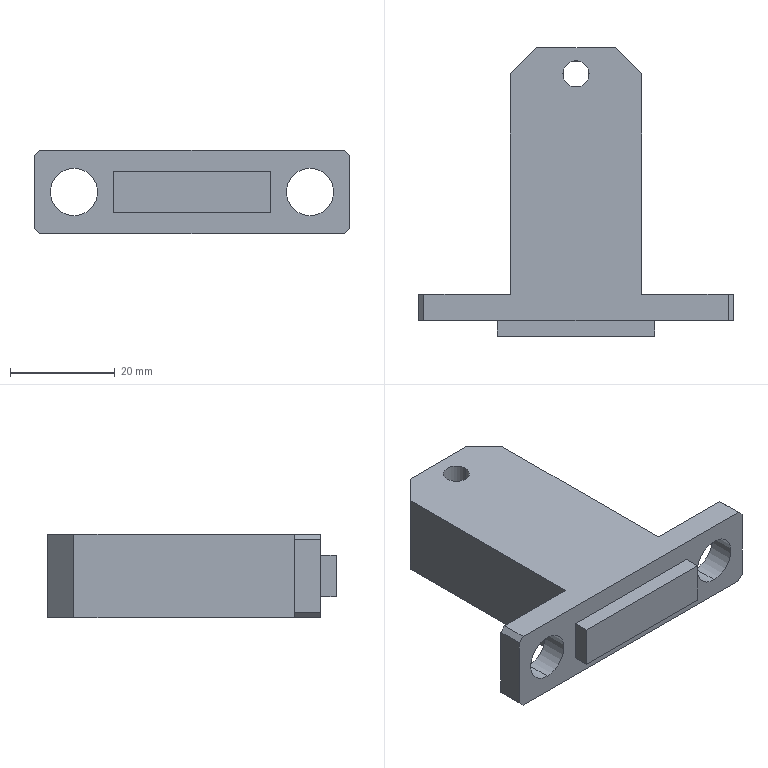Part | SolidWorks | features BaseBody 1 | 1 solid | 27 faces | box 60 x 55 x 16 mm | volume 22960 mm3 | plane 21 | cylinder 6 | commonest cylinder face diameters 9 x4 5 x2
STEP:
#1=CARTESIAN_POINT('',(-2.5,50.,-8.));
#2=VERTEX_POINT('',#1);
#3=CARTESIAN_POINT('',(2.5,50.,-8.));
#4=VERTEX_POINT('',#3);
#5=CARTESIAN_POINT('',(0.,50.,-8.));
#6=DIRECTION('',(0.,0.,1.));
#7=DIRECTION('',(1.,0.,0.));
#8=AXIS2_PLACEMENT_3D('',#5,#6,#7);
#9=CIRCLE('',#8,2.5);
#10=EDGE_CURVE('',#2,#4,#9,.T.);
#11=ORIENTED_EDGE('',*,*,#10,.F.);
#12=CARTESIAN_POINT('',(-2.5,50.,8.));
#13=VERTEX_POINT('',#12);
#14=CARTESIAN_POINT('',(-2.5,50.,8.));
#15=DIRECTION('',(0.,0.,1.));
#16=VECTOR('',#15,1000.);
#17=LINE('',#14,#16);
#18=EDGE_CURVE('',#2,#13,#17,.T.);
#19=ORIENTED_EDGE('',*,*,#18,.T.);
#20=CARTESIAN_POINT('',(2.5,50.,8.));
#21=VERTEX_POINT('',#20);
#22=CARTESIAN_POINT('',(0.,50.,8.));
#23=DIRECTION('',(0.,0.,1.));
#24=DIRECTION('',(1.,0.,0.));
#25=AXIS2_PLACEMENT_3D('',#22,#23,#24);
#26=CIRCLE('',#25,2.5);
#27=EDGE_CURVE('',#13,#21,#26,.T.);
#28=ORIENTED_EDGE('',*,*,#27,.T.);
#29=CARTESIAN_POINT('',(2.5,50.,8.));
#30=DIRECTION('',(0.,0.,1.));
#31=VECTOR('',#30,1000.);
#32=LINE('',#29,#31);
#33=EDGE_CURVE('',#4,#21,#32,.T.);
#34=ORIENTED_EDGE('',*,*,#33,.F.);
#35=EDGE_LOOP('',(#11,#19,#28,#34));
#36=FACE_OUTER_BOUND('',#35,.T.);
#37=CARTESIAN_POINT('',(0.,50.,8.));
#38=DIRECTION('',(0.,0.,1.));
#39=DIRECTION('',(1.,0.,0.));
#40=AXIS2_PLACEMENT_3D('',#37,#38,#39);
#41=CYLINDRICAL_SURFACE('',#40,2.5);
#42=ADVANCED_FACE('',(#36),#41,.F.);
#43=CARTESIAN_POINT('',(-22.5,3.,4.5));
#44=VERTEX_POINT('',#43);
#45=CARTESIAN_POINT('',(-22.5,3.,-4.5));
#46=VERTEX_POINT('',#45);
#47=CARTESIAN_POINT('',(-22.5,3.,0.));
#48=DIRECTION('',(0.,-1.,0.));
#49=DIRECTION('',(0.,0.,-1.));
#50=AXIS2_PLACEMENT_3D('',#47,#48,#49);
#51=CIRCLE('',#50,4.5);
#52=EDGE_CURVE('',#44,#46,#51,.T.);
#53=ORIENTED_EDGE('',*,*,#52,.T.);
#54=CARTESIAN_POINT('',(-22.5,8.,-4.5));
#55=VERTEX_POINT('',#54);
#56=CARTESIAN_POINT('',(-22.5,8.,-4.5));
#57=DIRECTION('',(0.,1.,0.));
#58=VECTOR('',#57,1000.);
#59=LINE('',#56,#58);
#60=EDGE_CURVE('',#46,#55,#59,.T.);
#61=ORIENTED_EDGE('',*,*,#60,.T.);
#62=CARTESIAN_POINT('',(-22.5,8.,4.5));
#63=VERTEX_POINT('',#62);
#64=CARTESIAN_POINT('',(-22.5,8.,0.));
#65=DIRECTION('',(0.,1.,0.));
#66=DIRECTION('',(0.,0.,1.));
#67=AXIS2_PLACEMENT_3D('',#64,#65,#66);
#68=CIRCLE('',#67,4.5);
#69=EDGE_CURVE('',#55,#63,#68,.T.);
#70=ORIENTED_EDGE('',*,*,#69,.T.);
#71=CARTESIAN_POINT('',(-22.5,8.,4.5));
#72=DIRECTION('',(0.,1.,0.));
#73=VECTOR('',#72,1000.);
#74=LINE('',#71,#73);
#75=EDGE_CURVE('',#44,#63,#74,.T.);
#76=ORIENTED_EDGE('',*,*,#75,.F.);
#77=EDGE_LOOP('',(#53,#61,#70,#76));
#78=FACE_OUTER_BOUND('',#77,.T.);
#79=CARTESIAN_POINT('',(-22.5,8.,0.));
#80=DIRECTION('',(0.,1.,0.));
#81=DIRECTION('',(0.,0.,1.));
#82=AXIS2_PLACEMENT_3D('',#79,#80,#81);
#83=CYLINDRICAL_SURFACE('',#82,4.5);
#84=ADVANCED_FACE('',(#78),#83,.F.);
#85=CARTESIAN_POINT('',(22.5,3.,4.5));
#86=VERTEX_POINT('',#85);
#87=CARTESIAN_POINT('',(22.5,3.,-4.5));
#88=VERTEX_POINT('',#87);
#89=CARTESIAN_POINT('',(22.5,3.,0.));
#90=DIRECTION('',(0.,-1.,0.));
#91=DIRECTION('',(0.,0.,-1.));
#92=AXIS2_PLACEMENT_3D('',#89,#90,#91);
#93=CIRCLE('',#92,4.5);
#94=EDGE_CURVE('',#86,#88,#93,.T.);
#95=ORIENTED_EDGE('',*,*,#94,.T.);
#96=CARTESIAN_POINT('',(22.5,8.,-4.5));
#97=VERTEX_POINT('',#96);
#98=CARTESIAN_POINT('',(22.5,8.,-4.5));
#99=DIRECTION('',(0.,1.,0.));
#100=VECTOR('',#99,1000.);
#101=LINE('',#98,#100);
#102=EDGE_CURVE('',#88,#97,#101,.T.);
#103=ORIENTED_EDGE('',*,*,#102,.T.);
#104=CARTESIAN_POINT('',(22.5,8.,4.5));
#105=VERTEX_POINT('',#104);
#106=CARTESIAN_POINT('',(22.5,8.,0.));
#107=DIRECTION('',(0.,1.,0.));
#108=DIRECTION('',(0.,0.,1.));
#109=AXIS2_PLACEMENT_3D('',#106,#107,#108);
#110=CIRCLE('',#109,4.5);
#111=EDGE_CURVE('',#97,#105,#110,.T.);
#112=ORIENTED_EDGE('',*,*,#111,.T.);
#113=CARTESIAN_POINT('',(22.5,8.,4.5));
#114=DIRECTION('',(0.,1.,0.));
#115=VECTOR('',#114,1000.);
#116=LINE('',#113,#115);
#117=EDGE_CURVE('',#86,#105,#116,.T.);
#118=ORIENTED_EDGE('',*,*,#117,.F.);
#119=EDGE_LOOP('',(#95,#103,#112,#118));
#120=FACE_OUTER_BOUND('',#119,.T.);
#121=CARTESIAN_POINT('',(22.5,8.,0.));
#122=DIRECTION('',(0.,1.,0.));
#123=DIRECTION('',(0.,0.,1.));
#124=AXIS2_PLACEMENT_3D('',#121,#122,#123);
#125=CYLINDRICAL_SURFACE('',#124,4.5);
#126=ADVANCED_FACE('',(#120),#125,.F.);
#127=CARTESIAN_POINT('',(29.,3.,8.));
#128=VERTEX_POINT('',#127);
#129=CARTESIAN_POINT('',(-29.,3.,8.));
#130=VERTEX_POINT('',#129);
#131=CARTESIAN_POINT('',(-30.,3.,8.));
#132=DIRECTION('',(-1.,0.,0.));
#133=VECTOR('',#132,1000.);
#134=LINE('',#131,#133);
#135=EDGE_CURVE('',#128,#130,#134,.T.);
#136=ORIENTED_EDGE('',*,*,#135,.F.);
#137=CARTESIAN_POINT('',(29.,8.,8.));
#138=VERTEX_POINT('',#137);
#139=CARTESIAN_POINT('',(29.,55.,8.));
#140=DIRECTION('',(0.,1.,0.));
#141=VECTOR('',#140,1000.);
#142=LINE('',#139,#141);
#143=EDGE_CURVE('',#128,#138,#142,.T.);
#144=ORIENTED_EDGE('',*,*,#143,.T.);
#145=CARTESIAN_POINT('',(12.5,8.,8.));
#146=VERTEX_POINT('',#145);
#147=CARTESIAN_POINT('',(30.,8.,8.));
#148=DIRECTION('',(1.,0.,0.));
#149=VECTOR('',#148,1000.);
#150=LINE('',#147,#149);
#151=EDGE_CURVE('',#146,#138,#150,.T.);
#152=ORIENTED_EDGE('',*,*,#151,.F.);
#153=CARTESIAN_POINT('',(12.5,50.,8.));
#154=VERTEX_POINT('',#153);
#155=CARTESIAN_POINT('',(12.5,55.,8.));
#156=DIRECTION('',(0.,-1.,0.));
#157=VECTOR('',#156,1000.);
#158=LINE('',#155,#157);
#159=EDGE_CURVE('',#154,#146,#158,.T.);
#160=ORIENTED_EDGE('',*,*,#159,.F.);
#161=CARTESIAN_POINT('',(7.5,55.,8.));
#162=VERTEX_POINT('',#161);
#163=CARTESIAN_POINT('',(12.5,50.,8.));
#164=DIRECTION('',(-0.7071,0.7071,0.));
#165=VECTOR('',#164,1000.);
#166=LINE('',#163,#165);
#167=EDGE_CURVE('',#154,#162,#166,.T.);
#168=ORIENTED_EDGE('',*,*,#167,.T.);
#169=CARTESIAN_POINT('',(-7.5,55.,8.));
#170=VERTEX_POINT('',#169);
#171=CARTESIAN_POINT('',(30.,55.,8.));
#172=DIRECTION('',(1.,0.,0.));
#173=VECTOR('',#172,1000.);
#174=LINE('',#171,#173);
#175=EDGE_CURVE('',#170,#162,#174,.T.);
#176=ORIENTED_EDGE('',*,*,#175,.F.);
#177=CARTESIAN_POINT('',(-12.5,50.,8.));
#178=VERTEX_POINT('',#177);
#179=CARTESIAN_POINT('',(-7.5,55.,8.));
#180=DIRECTION('',(-0.7071,-0.7071,0.));
#181=VECTOR('',#180,1000.);
#182=LINE('',#179,#181);
#183=EDGE_CURVE('',#170,#178,#182,.T.);
#184=ORIENTED_EDGE('',*,*,#183,.T.);
#185=CARTESIAN_POINT('',(-12.5,8.,8.));
#186=VERTEX_POINT('',#185);
#187=CARTESIAN_POINT('',(-12.5,55.,8.));
#188=DIRECTION('',(0.,1.,0.));
#189=VECTOR('',#188,1000.);
#190=LINE('',#187,#189);
#191=EDGE_CURVE('',#186,#178,#190,.T.);
#192=ORIENTED_EDGE('',*,*,#191,.F.);
#193=CARTESIAN_POINT('',(-29.,8.,8.));
#194=VERTEX_POINT('',#193);
#195=CARTESIAN_POINT('',(-30.,8.,8.));
#196=DIRECTION('',(1.,0.,0.));
#197=VECTOR('',#196,1000.);
#198=LINE('',#195,#197);
#199=EDGE_CURVE('',#194,#186,#198,.T.);
#200=ORIENTED_EDGE('',*,*,#199,.F.);
#201=CARTESIAN_POINT('',(-29.,55.,8.));
#202=DIRECTION('',(0.,-1.,0.));
#203=VECTOR('',#202,1000.);
#204=LINE('',#201,#203);
#205=EDGE_CURVE('',#194,#130,#204,.T.);
#206=ORIENTED_EDGE('',*,*,#205,.T.);
#207=EDGE_LOOP('',(#136,#144,#152,#160,#168,#176,#184,#192,#200,#206));
#208=FACE_OUTER_BOUND('',#207,.T.);
#209=CARTESIAN_POINT('',(0.,50.,8.));
#210=DIRECTION('',(0.,0.,1.));
#211=DIRECTION('',(1.,0.,0.));
#212=AXIS2_PLACEMENT_3D('',#209,#210,#211);
#213=CIRCLE('',#212,2.5);
#214=EDGE_CURVE('',#21,#13,#213,.T.);
#215=ORIENTED_EDGE('',*,*,#214,.F.);
#216=ORIENTED_EDGE('',*,*,#27,.F.);
#217=EDGE_LOOP('',(#215,#216));
#218=FACE_BOUND('',#217,.T.);
#219=CARTESIAN_POINT('',(30.,55.,8.));
#220=DIRECTION('',(0.,0.,-1.));
#221=DIRECTION('',(-1.,0.,0.));
#222=AXIS2_PLACEMENT_3D('',#219,#220,#221);
#223=PLANE('',#222);
#224=ADVANCED_FACE('',(#208,#218),#223,.F.);
#225=CARTESIAN_POINT('',(30.,3.,-7.));
#226=VERTEX_POINT('',#225);
#227=CARTESIAN_POINT('',(30.,3.,7.));
#228=VERTEX_POINT('',#227);
#229=CARTESIAN_POINT('',(30.,3.,8.));
#230=DIRECTION('',(0.,0.,1.));
#231=VECTOR('',#230,1000.);
#232=LINE('',#229,#231);
#233=EDGE_CURVE('',#226,#228,#232,.T.);
#234=ORIENTED_EDGE('',*,*,#233,.F.);
#235=CARTESIAN_POINT('',(30.,8.,-7.));
#236=VERTEX_POINT('',#235);
#237=CARTESIAN_POINT('',(30.,55.,-7.));
#238=DIRECTION('',(0.,1.,0.));
#239=VECTOR('',#238,1000.);
#240=LINE('',#237,#239);
#241=EDGE_CURVE('',#226,#236,#240,.T.);
#242=ORIENTED_EDGE('',*,*,#241,.T.);
#243=CARTESIAN_POINT('',(30.,8.,7.));
#244=VERTEX_POINT('',#243);
#245=CARTESIAN_POINT('',(30.,8.,-8.));
#246=DIRECTION('',(0.,0.,1.));
#247=VECTOR('',#246,1000.);
#248=LINE('',#245,#247);
#249=EDGE_CURVE('',#236,#244,#248,.T.);
#250=ORIENTED_EDGE('',*,*,#249,.T.);
#251=CARTESIAN_POINT('',(30.,55.,7.));
#252=DIRECTION('',(0.,-1.,0.));
#253=VECTOR('',#252,1000.);
#254=LINE('',#251,#253);
#255=EDGE_CURVE('',#244,#228,#254,.T.);
#256=ORIENTED_EDGE('',*,*,#255,.T.);
#257=EDGE_LOOP('',(#234,#242,#250,#256));
#258=FACE_OUTER_BOUND('',#257,.T.);
#259=CARTESIAN_POINT('',(30.,55.,-8.));
#260=DIRECTION('',(-1.,0.,0.));
#261=DIRECTION('',(0.,0.,1.));
#262=AXIS2_PLACEMENT_3D('',#259,#260,#261);
#263=PLANE('',#262);
#264=ADVANCED_FACE('',(#258),#263,.F.);
#265=ORIENTED_EDGE('',*,*,#102,.F.);
#266=CARTESIAN_POINT('',(22.5,3.,0.));
#267=DIRECTION('',(0.,-1.,0.));
#268=DIRECTION('',(0.,0.,-1.));
#269=AXIS2_PLACEMENT_3D('',#266,#267,#268);
#270=CIRCLE('',#269,4.5);
#271=EDGE_CURVE('',#88,#86,#270,.T.);
#272=ORIENTED_EDGE('',*,*,#271,.T.);
#273=ORIENTED_EDGE('',*,*,#117,.T.);
#274=CARTESIAN_POINT('',(22.5,8.,0.));
#275=DIRECTION('',(0.,1.,0.));
#276=DIRECTION('',(0.,0.,1.));
#277=AXIS2_PLACEMENT_3D('',#274,#275,#276);
#278=CIRCLE('',#277,4.5);
#279=EDGE_CURVE('',#105,#97,#278,.T.);
#280=ORIENTED_EDGE('',*,*,#279,.T.);
#281=EDGE_LOOP('',(#265,#272,#273,#280));
#282=FACE_OUTER_BOUND('',#281,.T.);
#283=CARTESIAN_POINT('',(22.5,8.,0.));
#284=DIRECTION('',(0.,1.,0.));
#285=DIRECTION('',(0.,0.,1.));
#286=AXIS2_PLACEMENT_3D('',#283,#284,#285);
#287=CYLINDRICAL_SURFACE('',#286,4.5);
#288=ADVANCED_FACE('',(#282),#287,.F.);
#289=CARTESIAN_POINT('',(-30.,3.,7.));
#290=VERTEX_POINT('',#289);
#291=CARTESIAN_POINT('',(-30.,3.,-7.));
#292=VERTEX_POINT('',#291);
#293=CARTESIAN_POINT('',(-30.,3.,-8.));
#294=DIRECTION('',(0.,0.,-1.));
#295=VECTOR('',#294,1000.);
#296=LINE('',#293,#295);
#297=EDGE_CURVE('',#290,#292,#296,.T.);
#298=ORIENTED_EDGE('',*,*,#297,.F.);
#299=CARTESIAN_POINT('',(-30.,8.,7.));
#300=VERTEX_POINT('',#299);
#301=CARTESIAN_POINT('',(-30.,55.,7.));
#302=DIRECTION('',(0.,1.,0.));
#303=VECTOR('',#302,1000.);
#304=LINE('',#301,#303);
#305=EDGE_CURVE('',#290,#300,#304,.T.);
#306=ORIENTED_EDGE('',*,*,#305,.T.);
#307=CARTESIAN_POINT('',(-30.,8.,-7.));
#308=VERTEX_POINT('',#307);
#309=CARTESIAN_POINT('',(-30.,8.,-8.));
#310=DIRECTION('',(0.,0.,1.));
#311=VECTOR('',#310,1000.);
#312=LINE('',#309,#311);
#313=EDGE_CURVE('',#308,#300,#312,.T.);
#314=ORIENTED_EDGE('',*,*,#313,.F.);
#315=CARTESIAN_POINT('',(-30.,55.,-7.));
#316=DIRECTION('',(0.,-1.,0.));
#317=VECTOR('',#316,1000.);
#318=LINE('',#315,#317);
#319=EDGE_CURVE('',#308,#292,#318,.T.);
#320=ORIENTED_EDGE('',*,*,#319,.T.);
#321=EDGE_LOOP('',(#298,#306,#314,#320));
#322=FACE_OUTER_BOUND('',#321,.T.);
#323=CARTESIAN_POINT('',(-30.,55.,-8.));
#324=DIRECTION('',(1.,0.,0.));
#325=DIRECTION('',(0.,0.,-1.));
#326=AXIS2_PLACEMENT_3D('',#323,#324,#325);
#327=PLANE('',#326);
#328=ADVANCED_FACE('',(#322),#327,.F.);
#329=ORIENTED_EDGE('',*,*,#60,.F.);
#330=CARTESIAN_POINT('',(-22.5,3.,0.));
#331=DIRECTION('',(0.,-1.,0.));
#332=DIRECTION('',(0.,0.,-1.));
#333=AXIS2_PLACEMENT_3D('',#330,#331,#332);
#334=CIRCLE('',#333,4.5);
#335=EDGE_CURVE('',#46,#44,#334,.T.);
#336=ORIENTED_EDGE('',*,*,#335,.T.);
#337=ORIENTED_EDGE('',*,*,#75,.T.);
#338=CARTESIAN_POINT('',(-22.5,8.,0.));
#339=DIRECTION('',(0.,1.,0.));
#340=DIRECTION('',(0.,0.,1.));
#341=AXIS2_PLACEMENT_3D('',#338,#339,#340);
#342=CIRCLE('',#341,4.5);
#343=EDGE_CURVE('',#63,#55,#342,.T.);
#344=ORIENTED_EDGE('',*,*,#343,.T.);
#345=EDGE_LOOP('',(#329,#336,#337,#344));
#346=FACE_OUTER_BOUND('',#345,.T.);
#347=CARTESIAN_POINT('',(-22.5,8.,0.));
#348=DIRECTION('',(0.,1.,0.));
#349=DIRECTION('',(0.,0.,1.));
#350=AXIS2_PLACEMENT_3D('',#347,#348,#349);
#351=CYLINDRICAL_SURFACE('',#350,4.5);
#352=ADVANCED_FACE('',(#346),#351,.F.);
#353=CARTESIAN_POINT('',(15.,0.,4.));
#354=VERTEX_POINT('',#353);
#355=CARTESIAN_POINT('',(15.,0.,-4.));
#356=VERTEX_POINT('',#355);
#357=CARTESIAN_POINT('',(15.,0.,8.));
#358=DIRECTION('',(0.,0.,-1.));
#359=VECTOR('',#358,1000.);
#360=LINE('',#357,#359);
#361=EDGE_CURVE('',#354,#356,#360,.T.);
#362=ORIENTED_EDGE('',*,*,#361,.F.);
#363=CARTESIAN_POINT('',(-15.,0.,4.));
#364=VERTEX_POINT('',#363);
#365=CARTESIAN_POINT('',(-30.,0.,4.));
#366=DIRECTION('',(1.,0.,0.));
#367=VECTOR('',#366,1000.);
#368=LINE('',#365,#367);
#369=EDGE_CURVE('',#364,#354,#368,.T.);
#370=ORIENTED_EDGE('',*,*,#369,.F.);
#371=CARTESIAN_POINT('',(-15.,0.,-4.));
#372=VERTEX_POINT('',#371);
#373=CARTESIAN_POINT('',(-15.,0.,8.));
#374=DIRECTION('',(0.,0.,1.));
#375=VECTOR('',#374,1000.);
#376=LINE('',#373,#375);
#377=EDGE_CURVE('',#372,#364,#376,.T.);
#378=ORIENTED_EDGE('',*,*,#377,.F.);
#379=CARTESIAN_POINT('',(-30.,0.,-4.));
#380=DIRECTION('',(-1.,0.,0.));
#381=VECTOR('',#380,1000.);
#382=LINE('',#379,#381);
#383=EDGE_CURVE('',#356,#372,#382,.T.);
#384=ORIENTED_EDGE('',*,*,#383,.F.);
#385=EDGE_LOOP('',(#362,#370,#378,#384));
#386=FACE_OUTER_BOUND('',#385,.T.);
#387=CARTESIAN_POINT('',(0.,0.,0.));
#388=DIRECTION('',(0.,-1.,0.));
#389=DIRECTION('',(0.,0.,-1.));
#390=AXIS2_PLACEMENT_3D('',#387,#388,#389);
#391=PLANE('',#390);
#392=ADVANCED_FACE('',(#386),#391,.T.);
#393=CARTESIAN_POINT('',(15.,3.,-4.));
#394=VERTEX_POINT('',#393);
#395=CARTESIAN_POINT('',(-15.,3.,-4.));
#396=VERTEX_POINT('',#395);
#397=CARTESIAN_POINT('',(-30.,3.,-4.));
#398=DIRECTION('',(-1.,0.,0.));
#399=VECTOR('',#398,1000.);
#400=LINE('',#397,#399);
#401=EDGE_CURVE('',#394,#396,#400,.T.);
#402=ORIENTED_EDGE('',*,*,#401,.F.);
#403=CARTESIAN_POINT('',(15.,3.,-4.));
#404=DIRECTION('',(0.,-1.,0.));
#405=VECTOR('',#404,1000.);
#406=LINE('',#403,#405);
#407=EDGE_CURVE('',#394,#356,#406,.T.);
#408=ORIENTED_EDGE('',*,*,#407,.T.);
#409=ORIENTED_EDGE('',*,*,#383,.T.);
#410=CARTESIAN_POINT('',(-15.,3.,-4.));
#411=DIRECTION('',(0.,1.,0.));
#412=VECTOR('',#411,1000.);
#413=LINE('',#410,#412);
#414=EDGE_CURVE('',#372,#396,#413,.T.);
#415=ORIENTED_EDGE('',*,*,#414,.T.);
#416=EDGE_LOOP('',(#402,#408,#409,#415));
#417=FACE_OUTER_BOUND('',#416,.T.);
#418=CARTESIAN_POINT('',(-30.,3.,-4.));
#419=DIRECTION('',(0.,0.,1.));
#420=DIRECTION('',(1.,0.,0.));
#421=AXIS2_PLACEMENT_3D('',#418,#419,#420);
#422=PLANE('',#421);
#423=ADVANCED_FACE('',(#417),#422,.F.);
#424=ORIENTED_EDGE('',*,*,#369,.T.);
#425=CARTESIAN_POINT('',(15.,3.,4.));
#426=VERTEX_POINT('',#425);
#427=CARTESIAN_POINT('',(15.,3.,4.));
#428=DIRECTION('',(0.,1.,0.));
#429=VECTOR('',#428,1000.);
#430=LINE('',#427,#429);
#431=EDGE_CURVE('',#354,#426,#430,.T.);
#432=ORIENTED_EDGE('',*,*,#431,.T.);
#433=CARTESIAN_POINT('',(-15.,3.,4.));
#434=VERTEX_POINT('',#433);
#435=CARTESIAN_POINT('',(-30.,3.,4.));
#436=DIRECTION('',(1.,0.,0.));
#437=VECTOR('',#436,1000.);
#438=LINE('',#435,#437);
#439=EDGE_CURVE('',#434,#426,#438,.T.);
#440=ORIENTED_EDGE('',*,*,#439,.F.);
#441=CARTESIAN_POINT('',(-15.,3.,4.));
#442=DIRECTION('',(0.,-1.,0.));
#443=VECTOR('',#442,1000.);
#444=LINE('',#441,#443);
#445=EDGE_CURVE('',#434,#364,#444,.T.);
#446=ORIENTED_EDGE('',*,*,#445,.T.);
#447=EDGE_LOOP('',(#424,#432,#440,#446));
#448=FACE_OUTER_BOUND('',#447,.T.);
#449=CARTESIAN_POINT('',(-30.,3.,4.));
#450=DIRECTION('',(0.,0.,-1.));
#451=DIRECTION('',(-1.,0.,0.));
#452=AXIS2_PLACEMENT_3D('',#449,#450,#451);
#453=PLANE('',#452);
#454=ADVANCED_FACE('',(#448),#453,.F.);
#455=CARTESIAN_POINT('',(0.,50.,-8.));
#456=DIRECTION('',(0.,0.,1.));
#457=DIRECTION('',(1.,0.,0.));
#458=AXIS2_PLACEMENT_3D('',#455,#456,#457);
#459=CIRCLE('',#458,2.5);
#460=EDGE_CURVE('',#4,#2,#459,.T.);
#461=ORIENTED_EDGE('',*,*,#460,.T.);
#462=ORIENTED_EDGE('',*,*,#10,.T.);
#463=EDGE_LOOP('',(#461,#462));
#464=FACE_BOUND('',#463,.T.);
#465=CARTESIAN_POINT('',(12.5,8.,-8.));
#466=VERTEX_POINT('',#465);
#467=CARTESIAN_POINT('',(29.,8.,-8.));
#468=VERTEX_POINT('',#467);
#469=CARTESIAN_POINT('',(30.,8.,-8.));
#470=DIRECTION('',(1.,0.,0.));
#471=VECTOR('',#470,1000.);
#472=LINE('',#469,#471);
#473=EDGE_CURVE('',#466,#468,#472,.T.);
#474=ORIENTED_EDGE('',*,*,#473,.T.);
#475=CARTESIAN_POINT('',(29.,3.,-8.));
#476=VERTEX_POINT('',#475);
#477=CARTESIAN_POINT('',(29.,55.,-8.));
#478=DIRECTION('',(0.,-1.,0.));
#479=VECTOR('',#478,1000.);
#480=LINE('',#477,#479);
#481=EDGE_CURVE('',#468,#476,#480,.T.);
#482=ORIENTED_EDGE('',*,*,#481,.T.);
#483=CARTESIAN_POINT('',(-29.,3.,-8.));
#484=VERTEX_POINT('',#483);
#485=CARTESIAN_POINT('',(-30.,3.,-8.));
#486=DIRECTION('',(1.,0.,0.));
#487=VECTOR('',#486,1000.);
#488=LINE('',#485,#487);
#489=EDGE_CURVE('',#484,#476,#488,.T.);
#490=ORIENTED_EDGE('',*,*,#489,.F.);
#491=CARTESIAN_POINT('',(-29.,8.,-8.));
#492=VERTEX_POINT('',#491);
#493=CARTESIAN_POINT('',(-29.,55.,-8.));
#494=DIRECTION('',(0.,1.,0.));
#495=VECTOR('',#494,1000.);
#496=LINE('',#493,#495);
#497=EDGE_CURVE('',#484,#492,#496,.T.);
#498=ORIENTED_EDGE('',*,*,#497,.T.);
#499=CARTESIAN_POINT('',(-12.5,8.,-8.));
#500=VERTEX_POINT('',#499);
#501=CARTESIAN_POINT('',(-30.,8.,-8.));
#502=DIRECTION('',(1.,0.,0.));
#503=VECTOR('',#502,1000.);
#504=LINE('',#501,#503);
#505=EDGE_CURVE('',#492,#500,#504,.T.);
#506=ORIENTED_EDGE('',*,*,#505,.T.);
#507=CARTESIAN_POINT('',(-12.5,50.,-8.));
#508=VERTEX_POINT('',#507);
#509=CARTESIAN_POINT('',(-12.5,55.,-8.));
#510=DIRECTION('',(0.,1.,0.));
#511=VECTOR('',#510,1000.);
#512=LINE('',#509,#511);
#513=EDGE_CURVE('',#500,#508,#512,.T.);
#514=ORIENTED_EDGE('',*,*,#513,.T.);
#515=CARTESIAN_POINT('',(-7.5,55.,-8.));
#516=VERTEX_POINT('',#515);
#517=CARTESIAN_POINT('',(-7.5,55.,-8.));
#518=DIRECTION('',(0.7071,0.7071,0.));
#519=VECTOR('',#518,1000.);
#520=LINE('',#517,#519);
#521=EDGE_CURVE('',#508,#516,#520,.T.);
#522=ORIENTED_EDGE('',*,*,#521,.T.);
#523=CARTESIAN_POINT('',(7.5,55.,-8.));
#524=VERTEX_POINT('',#523);
#525=CARTESIAN_POINT('',(30.,55.,-8.));
#526=DIRECTION('',(-1.,0.,0.));
#527=VECTOR('',#526,1000.);
#528=LINE('',#525,#527);
#529=EDGE_CURVE('',#524,#516,#528,.T.);
#530=ORIENTED_EDGE('',*,*,#529,.F.);
#531=CARTESIAN_POINT('',(12.5,50.,-8.));
#532=VERTEX_POINT('',#531);
#533=CARTESIAN_POINT('',(12.5,50.,-8.));
#534=DIRECTION('',(0.7071,-0.7071,0.));
#535=VECTOR('',#534,1000.);
#536=LINE('',#533,#535);
#537=EDGE_CURVE('',#524,#532,#536,.T.);
#538=ORIENTED_EDGE('',*,*,#537,.T.);
#539=CARTESIAN_POINT('',(12.5,55.,-8.));
#540=DIRECTION('',(0.,-1.,0.));
#541=VECTOR('',#540,1000.);
#542=LINE('',#539,#541);
#543=EDGE_CURVE('',#532,#466,#542,.T.);
#544=ORIENTED_EDGE('',*,*,#543,.T.);
#545=EDGE_LOOP('',(#474,#482,#490,#498,#506,#514,#522,#530,#538,#544));
#546=FACE_OUTER_BOUND('',#545,.T.);
#547=CARTESIAN_POINT('',(30.,55.,-8.));
#548=DIRECTION('',(0.,0.,1.));
#549=DIRECTION('',(1.,0.,0.));
#550=AXIS2_PLACEMENT_3D('',#547,#548,#549);
#551=PLANE('',#550);
#552=ADVANCED_FACE('',(#464,#546),#551,.F.);
#553=ORIENTED_EDGE('',*,*,#175,.T.);
#554=CARTESIAN_POINT('',(7.5,55.,0.));
#555=DIRECTION('',(0.,0.,-1.));
#556=VECTOR('',#555,1000.);
#557=LINE('',#554,#556);
#558=EDGE_CURVE('',#162,#524,#557,.T.);
#559=ORIENTED_EDGE('',*,*,#558,.T.);
#560=ORIENTED_EDGE('',*,*,#529,.T.);
#561=CARTESIAN_POINT('',(-7.5,55.,0.));
#562=DIRECTION('',(0.,0.,1.));
#563=VECTOR('',#562,1000.);
#564=LINE('',#561,#563);
#565=EDGE_CURVE('',#516,#170,#564,.T.);
#566=ORIENTED_EDGE('',*,*,#565,.T.);
#567=EDGE_LOOP('',(#553,#559,#560,#566));
#568=FACE_OUTER_BOUND('',#567,.T.);
#569=CARTESIAN_POINT('',(0.,55.,0.));
#570=DIRECTION('',(0.,-1.,0.));
#571=DIRECTION('',(0.,0.,-1.));
#572=AXIS2_PLACEMENT_3D('',#569,#570,#571);
#573=PLANE('',#572);
#574=ADVANCED_FACE('',(#568),#573,.F.);
#575=ORIENTED_EDGE('',*,*,#191,.T.);
#576=CARTESIAN_POINT('',(-12.5,50.,-8.));
#577=DIRECTION('',(0.,0.,-1.));
#578=VECTOR('',#577,1000.);
#579=LINE('',#576,#578);
#580=EDGE_CURVE('',#178,#508,#579,.T.);
#581=ORIENTED_EDGE('',*,*,#580,.T.);
#582=ORIENTED_EDGE('',*,*,#513,.F.);
#583=CARTESIAN_POINT('',(-12.5,8.,-8.));
#584=DIRECTION('',(0.,0.,1.));
#585=VECTOR('',#584,1000.);
#586=LINE('',#583,#585);
#587=EDGE_CURVE('',#500,#186,#586,.T.);
#588=ORIENTED_EDGE('',*,*,#587,.T.);
#589=EDGE_LOOP('',(#575,#581,#582,#588));
#590=FACE_OUTER_BOUND('',#589,.T.);
#591=CARTESIAN_POINT('',(-12.5,55.,-8.));
#592=DIRECTION('',(1.,0.,0.));
#593=DIRECTION('',(0.,1.,0.));
#594=AXIS2_PLACEMENT_3D('',#591,#592,#593);
#595=PLANE('',#594);
#596=ADVANCED_FACE('',(#590),#595,.F.);
#597=ORIENTED_EDGE('',*,*,#343,.F.);
#598=ORIENTED_EDGE('',*,*,#69,.F.);
#599=EDGE_LOOP('',(#597,#598));
#600=FACE_BOUND('',#599,.T.);
#601=ORIENTED_EDGE('',*,*,#313,.T.);
#602=CARTESIAN_POINT('',(-29.,8.,8.));
#603=DIRECTION('',(0.7071,0.,0.7071));
#604=VECTOR('',#603,1000.);
#605=LINE('',#602,#604);
#606=EDGE_CURVE('',#300,#194,#605,.T.);
#607=ORIENTED_EDGE('',*,*,#606,.T.);
#608=ORIENTED_EDGE('',*,*,#199,.T.);
#609=ORIENTED_EDGE('',*,*,#587,.F.);
#610=ORIENTED_EDGE('',*,*,#505,.F.);
#611=CARTESIAN_POINT('',(-30.,8.,-7.));
#612=DIRECTION('',(-0.7071,0.,0.7071));
#613=VECTOR('',#612,1000.);
#614=LINE('',#611,#613);
#615=EDGE_CURVE('',#492,#308,#614,.T.);
#616=ORIENTED_EDGE('',*,*,#615,.T.);
#617=EDGE_LOOP('',(#601,#607,#608,#609,#610,#616));
#618=FACE_OUTER_BOUND('',#617,.T.);
#619=CARTESIAN_POINT('',(-30.,8.,-8.));
#620=DIRECTION('',(0.,-1.,0.));
#621=DIRECTION('',(0.,0.,-1.));
#622=AXIS2_PLACEMENT_3D('',#619,#620,#621);
#623=PLANE('',#622);
#624=ADVANCED_FACE('',(#600,#618),#623,.F.);
#625=ORIENTED_EDGE('',*,*,#279,.F.);
#626=ORIENTED_EDGE('',*,*,#111,.F.);
#627=EDGE_LOOP('',(#625,#626));
#628=FACE_BOUND('',#627,.T.);
#629=ORIENTED_EDGE('',*,*,#249,.F.);
#630=CARTESIAN_POINT('',(29.,8.,-8.));
#631=DIRECTION('',(-0.7071,0.,-0.7071));
#632=VECTOR('',#631,1000.);
#633=LINE('',#630,#632);
#634=EDGE_CURVE('',#236,#468,#633,.T.);
#635=ORIENTED_EDGE('',*,*,#634,.T.);
#636=ORIENTED_EDGE('',*,*,#473,.F.);
#637=CARTESIAN_POINT('',(12.5,8.,-8.));
#638=DIRECTION('',(0.,0.,1.));
#639=VECTOR('',#638,1000.);
#640=LINE('',#637,#639);
#641=EDGE_CURVE('',#466,#146,#640,.T.);
#642=ORIENTED_EDGE('',*,*,#641,.T.);
#643=ORIENTED_EDGE('',*,*,#151,.T.);
#644=CARTESIAN_POINT('',(30.,8.,7.));
#645=DIRECTION('',(0.7071,0.,-0.7071));
#646=VECTOR('',#645,1000.);
#647=LINE('',#644,#646);
#648=EDGE_CURVE('',#138,#244,#647,.T.);
#649=ORIENTED_EDGE('',*,*,#648,.T.);
#650=EDGE_LOOP('',(#629,#635,#636,#642,#643,#649));
#651=FACE_OUTER_BOUND('',#650,.T.);
#652=CARTESIAN_POINT('',(30.,8.,-8.));
#653=DIRECTION('',(0.,-1.,0.));
#654=DIRECTION('',(0.,0.,-1.));
#655=AXIS2_PLACEMENT_3D('',#652,#653,#654);
#656=PLANE('',#655);
#657=ADVANCED_FACE('',(#628,#651),#656,.F.);
#658=ORIENTED_EDGE('',*,*,#543,.F.);
#659=CARTESIAN_POINT('',(12.5,50.,-8.));
#660=DIRECTION('',(0.,0.,1.));
#661=VECTOR('',#660,1000.);
#662=LINE('',#659,#661);
#663=EDGE_CURVE('',#532,#154,#662,.T.);
#664=ORIENTED_EDGE('',*,*,#663,.T.);
#665=ORIENTED_EDGE('',*,*,#159,.T.);
#666=ORIENTED_EDGE('',*,*,#641,.F.);
#667=EDGE_LOOP('',(#658,#664,#665,#666));
#668=FACE_OUTER_BOUND('',#667,.T.);
#669=CARTESIAN_POINT('',(12.5,55.,-8.));
#670=DIRECTION('',(-1.,0.,0.));
#671=DIRECTION('',(0.,-1.,0.));
#672=AXIS2_PLACEMENT_3D('',#669,#670,#671);
#673=PLANE('',#672);
#674=ADVANCED_FACE('',(#668),#673,.F.);
#675=ORIENTED_EDGE('',*,*,#537,.F.);
#676=ORIENTED_EDGE('',*,*,#558,.F.);
#677=ORIENTED_EDGE('',*,*,#167,.F.);
#678=ORIENTED_EDGE('',*,*,#663,.F.);
#679=EDGE_LOOP('',(#675,#676,#677,#678));
#680=FACE_OUTER_BOUND('',#679,.T.);
#681=CARTESIAN_POINT('',(12.5,50.,-8.));
#682=DIRECTION('',(-0.7071,-0.7071,0.));
#683=DIRECTION('',(0.,0.,1.));
#684=AXIS2_PLACEMENT_3D('',#681,#682,#683);
#685=PLANE('',#684);
#686=ADVANCED_FACE('',(#680),#685,.F.);
#687=ORIENTED_EDGE('',*,*,#521,.F.);
#688=ORIENTED_EDGE('',*,*,#580,.F.);
#689=ORIENTED_EDGE('',*,*,#183,.F.);
#690=ORIENTED_EDGE('',*,*,#565,.F.);
#691=EDGE_LOOP('',(#687,#688,#689,#690));
#692=FACE_OUTER_BOUND('',#691,.T.);
#693=CARTESIAN_POINT('',(-7.5,55.,0.));
#694=DIRECTION('',(0.7071,-0.7071,0.));
#695=DIRECTION('',(0.,0.,1.));
#696=AXIS2_PLACEMENT_3D('',#693,#694,#695);
#697=PLANE('',#696);
#698=ADVANCED_FACE('',(#692),#697,.F.);
#699=CARTESIAN_POINT('',(15.,3.,8.));
#700=DIRECTION('',(0.,0.,1.));
#701=VECTOR('',#700,1000.);
#702=LINE('',#699,#701);
#703=EDGE_CURVE('',#394,#426,#702,.T.);
#704=ORIENTED_EDGE('',*,*,#703,.F.);
#705=ORIENTED_EDGE('',*,*,#401,.T.);
#706=CARTESIAN_POINT('',(-15.,3.,8.));
#707=DIRECTION('',(0.,0.,-1.));
#708=VECTOR('',#707,1000.);
#709=LINE('',#706,#708);
#710=EDGE_CURVE('',#434,#396,#709,.T.);
#711=ORIENTED_EDGE('',*,*,#710,.F.);
#712=ORIENTED_EDGE('',*,*,#439,.T.);
#713=EDGE_LOOP('',(#704,#705,#711,#712));
#714=FACE_BOUND('',#713,.T.);
#715=ORIENTED_EDGE('',*,*,#94,.F.);
#716=ORIENTED_EDGE('',*,*,#271,.F.);
#717=EDGE_LOOP('',(#715,#716));
#718=FACE_BOUND('',#717,.T.);
#719=CARTESIAN_POINT('',(18.5,3.,-18.5));
#720=DIRECTION('',(0.7071,0.,0.7071));
#721=VECTOR('',#720,1000.);
#722=LINE('',#719,#721);
#723=EDGE_CURVE('',#476,#226,#722,.T.);
#724=ORIENTED_EDGE('',*,*,#723,.T.);
#725=ORIENTED_EDGE('',*,*,#233,.T.);
#726=CARTESIAN_POINT('',(18.5,3.,18.5));
#727=DIRECTION('',(-0.7071,0.,0.7071));
#728=VECTOR('',#727,1000.);
#729=LINE('',#726,#728);
#730=EDGE_CURVE('',#228,#128,#729,.T.);
#731=ORIENTED_EDGE('',*,*,#730,.T.);
#732=ORIENTED_EDGE('',*,*,#135,.T.);
#733=CARTESIAN_POINT('',(-18.5,3.,18.5));
#734=DIRECTION('',(-0.7071,0.,-0.7071));
#735=VECTOR('',#734,1000.);
#736=LINE('',#733,#735);
#737=EDGE_CURVE('',#130,#290,#736,.T.);
#738=ORIENTED_EDGE('',*,*,#737,.T.);
#739=ORIENTED_EDGE('',*,*,#297,.T.);
#740=CARTESIAN_POINT('',(-18.5,3.,-18.5));
#741=DIRECTION('',(0.7071,0.,-0.7071));
#742=VECTOR('',#741,1000.);
#743=LINE('',#740,#742);
#744=EDGE_CURVE('',#292,#484,#743,.T.);
#745=ORIENTED_EDGE('',*,*,#744,.T.);
#746=ORIENTED_EDGE('',*,*,#489,.T.);
#747=EDGE_LOOP('',(#724,#725,#731,#732,#738,#739,#745,#746));
#748=FACE_OUTER_BOUND('',#747,.T.);
#749=ORIENTED_EDGE('',*,*,#52,.F.);
#750=ORIENTED_EDGE('',*,*,#335,.F.);
#751=EDGE_LOOP('',(#749,#750));
#752=FACE_BOUND('',#751,.T.);
#753=CARTESIAN_POINT('',(0.,3.,0.));
#754=DIRECTION('',(0.,-1.,0.));
#755=DIRECTION('',(0.,0.,-1.));
#756=AXIS2_PLACEMENT_3D('',#753,#754,#755);
#757=PLANE('',#756);
#758=ADVANCED_FACE('',(#714,#718,#748,#752),#757,.T.);
#759=ORIENTED_EDGE('',*,*,#634,.F.);
#760=ORIENTED_EDGE('',*,*,#241,.F.);
#761=ORIENTED_EDGE('',*,*,#723,.F.);
#762=ORIENTED_EDGE('',*,*,#481,.F.);
#763=EDGE_LOOP('',(#759,#760,#761,#762));
#764=FACE_OUTER_BOUND('',#763,.T.);
#765=CARTESIAN_POINT('',(29.,55.,-8.));
#766=DIRECTION('',(-0.7071,0.,0.7071));
#767=DIRECTION('',(0.,-1.,0.));
#768=AXIS2_PLACEMENT_3D('',#765,#766,#767);
#769=PLANE('',#768);
#770=ADVANCED_FACE('',(#764),#769,.F.);
#771=ORIENTED_EDGE('',*,*,#648,.F.);
#772=ORIENTED_EDGE('',*,*,#143,.F.);
#773=ORIENTED_EDGE('',*,*,#730,.F.);
#774=ORIENTED_EDGE('',*,*,#255,.F.);
#775=EDGE_LOOP('',(#771,#772,#773,#774));
#776=FACE_OUTER_BOUND('',#775,.T.);
#777=CARTESIAN_POINT('',(30.,55.,7.));
#778=DIRECTION('',(-0.7071,0.,-0.7071));
#779=DIRECTION('',(0.,-1.,0.));
#780=AXIS2_PLACEMENT_3D('',#777,#778,#779);
#781=PLANE('',#780);
#782=ADVANCED_FACE('',(#776),#781,.F.);
#783=ORIENTED_EDGE('',*,*,#606,.F.);
#784=ORIENTED_EDGE('',*,*,#305,.F.);
#785=ORIENTED_EDGE('',*,*,#737,.F.);
#786=ORIENTED_EDGE('',*,*,#205,.F.);
#787=EDGE_LOOP('',(#783,#784,#785,#786));
#788=FACE_OUTER_BOUND('',#787,.T.);
#789=CARTESIAN_POINT('',(-29.,55.,8.));
#790=DIRECTION('',(0.7071,0.,-0.7071));
#791=DIRECTION('',(0.,-1.,0.));
#792=AXIS2_PLACEMENT_3D('',#789,#790,#791);
#793=PLANE('',#792);
#794=ADVANCED_FACE('',(#788),#793,.F.);
#795=ORIENTED_EDGE('',*,*,#615,.F.);
#796=ORIENTED_EDGE('',*,*,#497,.F.);
#797=ORIENTED_EDGE('',*,*,#744,.F.);
#798=ORIENTED_EDGE('',*,*,#319,.F.);
#799=EDGE_LOOP('',(#795,#796,#797,#798));
#800=FACE_OUTER_BOUND('',#799,.T.);
#801=CARTESIAN_POINT('',(-30.,55.,-7.));
#802=DIRECTION('',(0.7071,0.,0.7071));
#803=DIRECTION('',(0.,-1.,0.));
#804=AXIS2_PLACEMENT_3D('',#801,#802,#803);
#805=PLANE('',#804);
#806=ADVANCED_FACE('',(#800),#805,.F.);
#807=ORIENTED_EDGE('',*,*,#377,.T.);
#808=ORIENTED_EDGE('',*,*,#445,.F.);
#809=ORIENTED_EDGE('',*,*,#710,.T.);
#810=ORIENTED_EDGE('',*,*,#414,.F.);
#811=EDGE_LOOP('',(#807,#808,#809,#810));
#812=FACE_OUTER_BOUND('',#811,.T.);
#813=CARTESIAN_POINT('',(-15.,24.932,8.));
#814=DIRECTION('',(1.,0.,0.));
#815=DIRECTION('',(0.,0.,-1.));
#816=AXIS2_PLACEMENT_3D('',#813,#814,#815);
#817=PLANE('',#816);
#818=ADVANCED_FACE('',(#812),#817,.F.);
#819=ORIENTED_EDGE('',*,*,#703,.T.);
#820=ORIENTED_EDGE('',*,*,#431,.F.);
#821=ORIENTED_EDGE('',*,*,#361,.T.);
#822=ORIENTED_EDGE('',*,*,#407,.F.);
#823=EDGE_LOOP('',(#819,#820,#821,#822));
#824=FACE_OUTER_BOUND('',#823,.T.);
#825=CARTESIAN_POINT('',(15.,24.932,8.));
#826=DIRECTION('',(-1.,0.,0.));
#827=DIRECTION('',(0.,0.,1.));
#828=AXIS2_PLACEMENT_3D('',#825,#826,#827);
#829=PLANE('',#828);
#830=ADVANCED_FACE('',(#824),#829,.F.);
#831=ORIENTED_EDGE('',*,*,#18,.F.);
#832=ORIENTED_EDGE('',*,*,#460,.F.);
#833=ORIENTED_EDGE('',*,*,#33,.T.);
#834=ORIENTED_EDGE('',*,*,#214,.T.);
#835=EDGE_LOOP('',(#831,#832,#833,#834));
#836=FACE_OUTER_BOUND('',#835,.T.);
#837=CARTESIAN_POINT('',(0.,50.,8.));
#838=DIRECTION('',(0.,0.,1.));
#839=DIRECTION('',(1.,0.,0.));
#840=AXIS2_PLACEMENT_3D('',#837,#838,#839);
#841=CYLINDRICAL_SURFACE('',#840,2.5);
#842=ADVANCED_FACE('',(#836),#841,.F.);
#843=CLOSED_SHELL('',(#42,#84,#126,#224,#264,#288,#328,#352,#392,#423,#454,#552,#574,#596,#624,#657,#674,#686,#698,#758,#770,#782,#794,#806,#818,#830,#842));
#844=MANIFOLD_SOLID_BREP('',#843);
#845=CARTESIAN_POINT('',(0.,0.,0.));
#846=DIRECTION('',(0.,0.,1.));
#847=DIRECTION('',(1.,0.,0.));
#848=AXIS2_PLACEMENT_3D('',#845,#846,#847);
#849=(LENGTH_UNIT()NAMED_UNIT(*)SI_UNIT(.MILLI.,.METRE.));
#850=UNCERTAINTY_MEASURE_WITH_UNIT(LENGTH_MEASURE(0.00001),#849,'','');
#851=(NAMED_UNIT(*)PLANE_ANGLE_UNIT()SI_UNIT($,.RADIAN.));
#852=(NAMED_UNIT(*)SI_UNIT($,.STERADIAN.)SOLID_ANGLE_UNIT());
#853=(GEOMETRIC_REPRESENTATION_CONTEXT(3)GLOBAL_UNCERTAINTY_ASSIGNED_CONTEXT((#850))GLOBAL_UNIT_ASSIGNED_CONTEXT((#849,#851,#852))REPRESENTATION_CONTEXT('',''));
#854=ADVANCED_BREP_SHAPE_REPRESENTATION('',(#844,#848),#853);